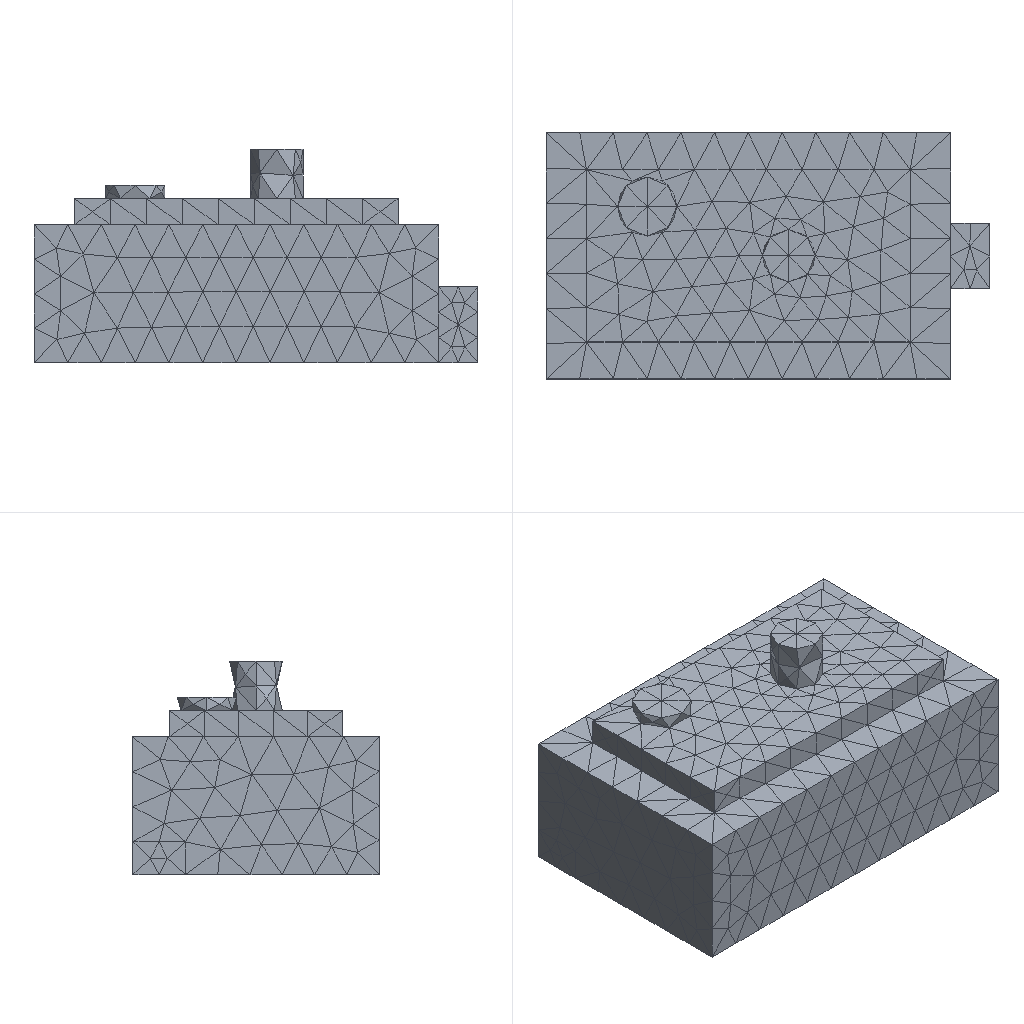Simulation study | ansys mapdl
Set-up summary:
category,name,step,type,value,unit,region
solver,ansys_mapdl
units,mm-N-s-tonne (MPa),,inferred,E=210000 density=
analysis,model,,static
mesh,nodes,,,5675
mesh,elements,,,3467
element_type,SOLID187,,,3467
material,mat 1,,E,210000
material,mat 1,,nu,0.3
load,,model,body load temp,,,all
load,,model,force,"1000 [dir=(0, 0, -1) n=140]",,node list
bc,,model,fixed,"[dofs=UX,UY,UZ n=6006]",,node list
Ansys APDL input file, long lists of numbers shortened:
/COM,ANSYS RELEASE 2026 R1           BUILD 26.1      UP20260202       09:11:09
/PREP7
/NOPR
/TITLE,2
ANTYPE, 0
*IF,_CDRDOFF,EQ,1,THEN     !if solid model was read in
_CDRDOFF=             !reset flag, numoffs already performed
*ELSE              !offset database for the following FE model
NUMOFF,NODE,     5675
NUMOFF,ELEM,     3467
NUMOFF,MAT ,        1
NUMOFF,TYPE,        1
*ENDIF
*SET,_RETURN ,  0.
*SET,_STATUS ,  0.
*SET,_UIQR   ,  140.
*SET,__FLOATPARAMETER__,  5675.
DOF,DELETE
ETBLOCK,        1,        1
(2i9,19a9)
        1      187        0        0        0        0        0        0        0        0        0        0        0        0        0        0        0        0        0        0        0
       -1
NBLOCK,6,SOLID,      5675,      5675
(3i9,6e21.13e3)
        1        0        0-4.5625000000000E+001 3.7500000000000E+001 1.0000000000000E+001
! (5674 more lines like these left out)
N,UNBL,LOC,       -1,
EBLOCK,19,SOLID,      3467,      3467
(19i10)
         1         1         1         1         0         0         0         0        10         0         1      2007      1680      2008      2009      2358      2359      2360      2361
! (6933 more lines like these left out)
        -1
MPTEMP,UNBL, 1, 1,  0.    ,
MPDATA,UNBL, 1,EX  ,       1, 1,  210000.000    ,
MPTEMP,UNBL, 1, 1,  0.    ,
MPDATA,UNBL, 1,NUXY,       1, 1, 0.3    ,
MPTEMP,UNBL, 1, 1,  0.    ,
MPDATA,UNBL, 1,PRXY,       1, 1, 0.3    ,
EXTOPT,ATTR,      0,      0,      0
EXTOPT,ESIZE,  0,  0.
EXTOPT,ACLEAR,      0
TREF,  0.
IRLF,  0
BFUNIF,TEMP,_TINY
ACEL,  0.    ,  0.    ,  0.
OMEGA,  0.    ,  0.    ,  0.
DOMEGA,  0.    ,  0.    ,  0.
CGLOC,  0.    ,  0.    ,  0.
CGOMEGA,  0.    ,  0.    ,  0.
DCGOMG,  0.    ,  0.    ,  0.
KUSE,     0
TIME,  0.
ALPHAD,  0.
BETAD,  0.
DMPRAT,  0.
DMPSTR,  0.
CRPLIM, 0.1    ,   0
CRPLIM,  0.    ,   1
NCNV,     0, 1.000000000E+12,     0,  0.    ,  0.
NEQIT,     0
ERESX,DEFA
DBLOCK,      6006
(i9,a6,2(pg16.9))
        1  UX    0.00000000      0.00000000
! (6005 more lines like these left out)
       -1
FBLOCK,       140
(i9,a6,2(pg16.9))
      948  FZ   -7.14285714      0.00000000
! (139 more lines like these left out)
       -1
/GO
FINISH
Results summary:
result,analysis_type_db,,,static,unstated
result,n_sets,,,1,unstated
result,load_steps[0].set,load_step=1,,1,unstated
result,load_steps[0].substep,load_step=1,,1,unstated
result,load_steps[0].time,load_step=1,,1,unstated
result,load_steps[0].freq,load_step=1,,1,unstated
result,load_steps[0].max_usum,load_step=1,,0.0004083,unstated
result,load_steps[0].max_seqv,load_step=1,,4.771,unstated
result,load_steps[0].reaction_sum.FX,load_step=1,,-1.10791e-11,unstated
result,load_steps[0].reaction_sum.FY,load_step=1,,-8.29203e-12,unstated
result,load_steps[0].reaction_sum.FZ,load_step=1,,1000,unstated
result,load_steps[0].reaction_sum.MX,load_step=1,,0,unstated
result,load_steps[0].reaction_sum.MY,load_step=1,,0,unstated
result,load_steps[0].reaction_sum.MZ,load_step=1,,0,unstated
result,convergence,,,results present for all listed sets,unstated